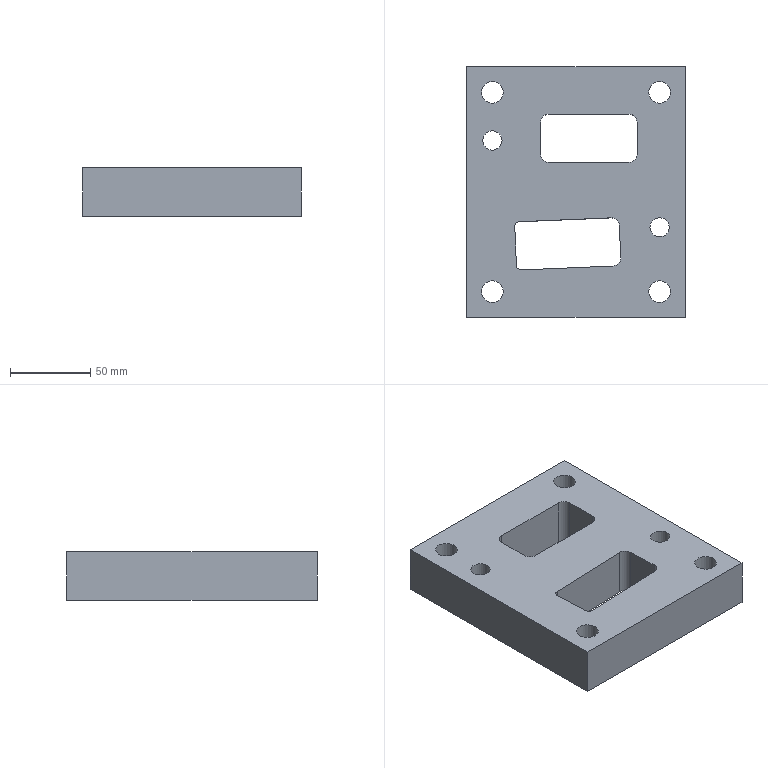Part | NX | features 7 2 | 1 solid | 40 faces | box 136 x 156 x 30 mm | volume 489972 mm3 | plane 20 | cylinder 20 | commonest cylinder face diameters 10 x6 13.5 x4 20 x4 6 x2 12.001 x2 14.11 x2
STEP:
#1=CARTESIAN_POINT('',(3690.489,357.828,91.));
#2=VERTEX_POINT('',#1);
#3=CARTESIAN_POINT('',(3693.361,360.951,91.));
#4=VERTEX_POINT('',#3);
#5=CARTESIAN_POINT('',(3693.487,357.953,91.));
#6=DIRECTION('',(0.,0.,-1.));
#7=DIRECTION('',(1.,0.,0.));
#8=AXIS2_PLACEMENT_3D('',#5,#6,#7);
#9=CIRCLE('',#8,3.);
#10=EDGE_CURVE('',#2,#4,#9,.T.);
#11=ORIENTED_EDGE('',*,*,#10,.T.);
#12=CARTESIAN_POINT('',(3750.311,363.335,91.));
#13=VERTEX_POINT('',#12);
#14=CARTESIAN_POINT('',(3740.376,362.919,91.));
#15=DIRECTION('',(-0.9991,-0.04184,0.));
#16=VECTOR('',#15,1000.);
#17=LINE('',#14,#16);
#18=EDGE_CURVE('',#13,#4,#17,.T.);
#19=ORIENTED_EDGE('',*,*,#18,.F.);
#20=CARTESIAN_POINT('',(3755.516,358.549,91.));
#21=VERTEX_POINT('',#20);
#22=CARTESIAN_POINT('',(3750.52,358.34,91.));
#23=DIRECTION('',(0.,0.,-1.));
#24=DIRECTION('',(1.,0.,0.));
#25=AXIS2_PLACEMENT_3D('',#22,#23,#24);
#26=CIRCLE('',#25,5.);
#27=EDGE_CURVE('',#13,#21,#26,.T.);
#28=ORIENTED_EDGE('',*,*,#27,.T.);
#29=CARTESIAN_POINT('',(3756.353,338.567,91.));
#30=VERTEX_POINT('',#29);
#31=CARTESIAN_POINT('',(3754.595,380.539,91.));
#32=DIRECTION('',(-0.04184,0.9991,0.));
#33=VECTOR('',#32,1000.);
#34=LINE('',#31,#33);
#35=EDGE_CURVE('',#30,#21,#34,.T.);
#36=ORIENTED_EDGE('',*,*,#35,.F.);
#37=CARTESIAN_POINT('',(3751.566,333.362,91.));
#38=VERTEX_POINT('',#37);
#39=CARTESIAN_POINT('',(3751.357,338.357,91.));
#40=DIRECTION('',(0.,0.,-1.));
#41=DIRECTION('',(1.,0.,0.));
#42=AXIS2_PLACEMENT_3D('',#39,#40,#41);
#43=CIRCLE('',#42,5.);
#44=EDGE_CURVE('',#30,#38,#43,.T.);
#45=ORIENTED_EDGE('',*,*,#44,.T.);
#46=CARTESIAN_POINT('',(3694.616,330.977,91.));
#47=VERTEX_POINT('',#46);
#48=CARTESIAN_POINT('',(3741.631,332.946,91.));
#49=DIRECTION('',(0.9991,0.04184,0.));
#50=VECTOR('',#49,1000.);
#51=LINE('',#48,#50);
#52=EDGE_CURVE('',#47,#38,#51,.T.);
#53=ORIENTED_EDGE('',*,*,#52,.F.);
#54=CARTESIAN_POINT('',(3691.493,333.849,91.));
#55=VERTEX_POINT('',#54);
#56=CARTESIAN_POINT('',(3694.491,333.974,91.));
#57=DIRECTION('',(0.,0.,-1.));
#58=DIRECTION('',(1.,0.,0.));
#59=AXIS2_PLACEMENT_3D('',#56,#57,#58);
#60=CIRCLE('',#59,3.);
#61=EDGE_CURVE('',#47,#55,#60,.T.);
#62=ORIENTED_EDGE('',*,*,#61,.T.);
#63=CARTESIAN_POINT('',(3689.652,377.82,91.));
#64=DIRECTION('',(0.04184,-0.9991,0.));
#65=VECTOR('',#64,1000.);
#66=LINE('',#63,#65);
#67=EDGE_CURVE('',#2,#55,#66,.T.);
#68=ORIENTED_EDGE('',*,*,#67,.F.);
#69=EDGE_LOOP('',(#11,#19,#28,#36,#45,#53,#62,#68));
#70=FACE_BOUND('',#69,.T.);
#71=CARTESIAN_POINT('',(3786.562,357.449,91.));
#72=VERTEX_POINT('',#71);
#73=CARTESIAN_POINT('',(3780.562,357.449,91.));
#74=DIRECTION('',(0.,0.,-1.));
#75=DIRECTION('',(1.,0.,0.));
#76=AXIS2_PLACEMENT_3D('',#73,#74,#75);
#77=CIRCLE('',#76,6.);
#78=EDGE_CURVE('',#72,#72,#77,.T.);
#79=ORIENTED_EDGE('',*,*,#78,.T.);
#80=EDGE_LOOP('',(#79));
#81=FACE_BOUND('',#80,.T.);
#82=CARTESIAN_POINT('',(3682.562,411.449,91.));
#83=VERTEX_POINT('',#82);
#84=CARTESIAN_POINT('',(3676.562,411.449,91.));
#85=DIRECTION('',(0.,0.,-1.));
#86=DIRECTION('',(1.,0.,0.));
#87=AXIS2_PLACEMENT_3D('',#84,#85,#86);
#88=CIRCLE('',#87,6.);
#89=EDGE_CURVE('',#83,#83,#88,.T.);
#90=ORIENTED_EDGE('',*,*,#89,.T.);
#91=EDGE_LOOP('',(#90));
#92=FACE_BOUND('',#91,.T.);
#93=CARTESIAN_POINT('',(3683.312,317.449,91.));
#94=VERTEX_POINT('',#93);
#95=CARTESIAN_POINT('',(3676.562,317.449,91.));
#96=DIRECTION('',(0.,0.,-1.));
#97=DIRECTION('',(1.,0.,0.));
#98=AXIS2_PLACEMENT_3D('',#95,#96,#97);
#99=CIRCLE('',#98,6.75);
#100=EDGE_CURVE('',#94,#94,#99,.T.);
#101=ORIENTED_EDGE('',*,*,#100,.T.);
#102=EDGE_LOOP('',(#101));
#103=FACE_BOUND('',#102,.T.);
#104=CARTESIAN_POINT('',(3787.312,441.449,91.));
#105=VERTEX_POINT('',#104);
#106=CARTESIAN_POINT('',(3780.562,441.449,91.));
#107=DIRECTION('',(0.,0.,-1.));
#108=DIRECTION('',(1.,0.,0.));
#109=AXIS2_PLACEMENT_3D('',#106,#107,#108);
#110=CIRCLE('',#109,6.75);
#111=EDGE_CURVE('',#105,#105,#110,.T.);
#112=ORIENTED_EDGE('',*,*,#111,.T.);
#113=EDGE_LOOP('',(#112));
#114=FACE_BOUND('',#113,.T.);
#115=CARTESIAN_POINT('',(3787.312,317.449,91.));
#116=VERTEX_POINT('',#115);
#117=CARTESIAN_POINT('',(3780.562,317.449,91.));
#118=DIRECTION('',(0.,0.,-1.));
#119=DIRECTION('',(1.,0.,0.));
#120=AXIS2_PLACEMENT_3D('',#117,#118,#119);
#121=CIRCLE('',#120,6.75);
#122=EDGE_CURVE('',#116,#116,#121,.T.);
#123=ORIENTED_EDGE('',*,*,#122,.T.);
#124=EDGE_LOOP('',(#123));
#125=FACE_BOUND('',#124,.T.);
#126=CARTESIAN_POINT('',(3683.312,441.449,91.));
#127=VERTEX_POINT('',#126);
#128=CARTESIAN_POINT('',(3676.562,441.449,91.));
#129=DIRECTION('',(0.,0.,-1.));
#130=DIRECTION('',(1.,0.,0.));
#131=AXIS2_PLACEMENT_3D('',#128,#129,#130);
#132=CIRCLE('',#131,6.75);
#133=EDGE_CURVE('',#127,#127,#132,.T.);
#134=ORIENTED_EDGE('',*,*,#133,.T.);
#135=EDGE_LOOP('',(#134));
#136=FACE_BOUND('',#135,.T.);
#137=CARTESIAN_POINT('',(3796.562,457.449,91.));
#138=VERTEX_POINT('',#137);
#139=CARTESIAN_POINT('',(3660.562,457.449,91.));
#140=VERTEX_POINT('',#139);
#141=CARTESIAN_POINT('',(3728.562,457.449,91.));
#142=DIRECTION('',(-1.,0.,0.));
#143=VECTOR('',#142,1000.);
#144=LINE('',#141,#143);
#145=EDGE_CURVE('',#138,#140,#144,.T.);
#146=ORIENTED_EDGE('',*,*,#145,.T.);
#147=CARTESIAN_POINT('',(3660.562,301.449,91.));
#148=VERTEX_POINT('',#147);
#149=CARTESIAN_POINT('',(3660.562,379.449,91.));
#150=DIRECTION('',(0.,-1.,0.));
#151=VECTOR('',#150,1000.);
#152=LINE('',#149,#151);
#153=EDGE_CURVE('',#140,#148,#152,.T.);
#154=ORIENTED_EDGE('',*,*,#153,.T.);
#155=CARTESIAN_POINT('',(3796.562,301.449,91.));
#156=VERTEX_POINT('',#155);
#157=CARTESIAN_POINT('',(3728.562,301.449,91.));
#158=DIRECTION('',(1.,0.,0.));
#159=VECTOR('',#158,1000.);
#160=LINE('',#157,#159);
#161=EDGE_CURVE('',#148,#156,#160,.T.);
#162=ORIENTED_EDGE('',*,*,#161,.T.);
#163=CARTESIAN_POINT('',(3796.562,379.449,91.));
#164=DIRECTION('',(0.,1.,0.));
#165=VECTOR('',#164,1000.);
#166=LINE('',#163,#165);
#167=EDGE_CURVE('',#156,#138,#166,.T.);
#168=ORIENTED_EDGE('',*,*,#167,.T.);
#169=EDGE_LOOP('',(#146,#154,#162,#168));
#170=FACE_BOUND('',#169,.T.);
#171=CARTESIAN_POINT('',(3711.499,397.84,91.));
#172=VERTEX_POINT('',#171);
#173=CARTESIAN_POINT('',(3706.499,402.84,91.));
#174=VERTEX_POINT('',#173);
#175=CARTESIAN_POINT('',(3711.499,402.84,91.));
#176=DIRECTION('',(0.,0.,-1.));
#177=DIRECTION('',(1.,0.,0.));
#178=AXIS2_PLACEMENT_3D('',#175,#176,#177);
#179=CIRCLE('',#178,5.);
#180=EDGE_CURVE('',#172,#174,#179,.T.);
#181=ORIENTED_EDGE('',*,*,#180,.T.);
#182=CARTESIAN_POINT('',(3706.499,422.84,91.));
#183=VERTEX_POINT('',#182);
#184=CARTESIAN_POINT('',(3706.499,412.84,91.));
#185=DIRECTION('',(0.,-1.,0.));
#186=VECTOR('',#185,1000.);
#187=LINE('',#184,#186);
#188=EDGE_CURVE('',#183,#174,#187,.T.);
#189=ORIENTED_EDGE('',*,*,#188,.F.);
#190=CARTESIAN_POINT('',(3711.499,427.84,91.));
#191=VERTEX_POINT('',#190);
#192=CARTESIAN_POINT('',(3711.499,422.84,91.));
#193=DIRECTION('',(0.,0.,-1.));
#194=DIRECTION('',(1.,0.,0.));
#195=AXIS2_PLACEMENT_3D('',#192,#193,#194);
#196=CIRCLE('',#195,5.);
#197=EDGE_CURVE('',#183,#191,#196,.T.);
#198=ORIENTED_EDGE('',*,*,#197,.T.);
#199=CARTESIAN_POINT('',(3761.499,427.84,91.));
#200=VERTEX_POINT('',#199);
#201=CARTESIAN_POINT('',(3721.499,427.84,91.));
#202=DIRECTION('',(-1.,0.,0.));
#203=VECTOR('',#202,1000.);
#204=LINE('',#201,#203);
#205=EDGE_CURVE('',#200,#191,#204,.T.);
#206=ORIENTED_EDGE('',*,*,#205,.F.);
#207=CARTESIAN_POINT('',(3766.499,422.84,91.));
#208=VERTEX_POINT('',#207);
#209=CARTESIAN_POINT('',(3761.499,422.84,91.));
#210=DIRECTION('',(0.,0.,-1.));
#211=DIRECTION('',(1.,0.,0.));
#212=AXIS2_PLACEMENT_3D('',#209,#210,#211);
#213=CIRCLE('',#212,5.);
#214=EDGE_CURVE('',#200,#208,#213,.T.);
#215=ORIENTED_EDGE('',*,*,#214,.T.);
#216=CARTESIAN_POINT('',(3766.499,402.84,91.));
#217=VERTEX_POINT('',#216);
#218=CARTESIAN_POINT('',(3766.499,412.84,91.));
#219=DIRECTION('',(0.,1.,0.));
#220=VECTOR('',#219,1000.);
#221=LINE('',#218,#220);
#222=EDGE_CURVE('',#217,#208,#221,.T.);
#223=ORIENTED_EDGE('',*,*,#222,.F.);
#224=CARTESIAN_POINT('',(3761.499,397.84,91.));
#225=VERTEX_POINT('',#224);
#226=CARTESIAN_POINT('',(3761.499,402.84,91.));
#227=DIRECTION('',(0.,0.,-1.));
#228=DIRECTION('',(1.,0.,0.));
#229=AXIS2_PLACEMENT_3D('',#226,#227,#228);
#230=CIRCLE('',#229,5.);
#231=EDGE_CURVE('',#217,#225,#230,.T.);
#232=ORIENTED_EDGE('',*,*,#231,.T.);
#233=CARTESIAN_POINT('',(3721.499,397.84,91.));
#234=DIRECTION('',(1.,0.,0.));
#235=VECTOR('',#234,1000.);
#236=LINE('',#233,#235);
#237=EDGE_CURVE('',#172,#225,#236,.T.);
#238=ORIENTED_EDGE('',*,*,#237,.F.);
#239=EDGE_LOOP('',(#181,#189,#198,#206,#215,#223,#232,#238));
#240=FACE_BOUND('',#239,.T.);
#241=CARTESIAN_POINT('',(3728.562,379.449,91.));
#242=DIRECTION('',(0.,0.,1.));
#243=DIRECTION('',(-1.,0.,0.));
#244=AXIS2_PLACEMENT_3D('',#241,#242,#243);
#245=PLANE('',#244);
#246=ADVANCED_FACE('',(#70,#81,#92,#103,#114,#125,#136,#170,#240),#245,.T.);
#247=CARTESIAN_POINT('',(3787.617,357.449,61.));
#248=VERTEX_POINT('',#247);
#249=CARTESIAN_POINT('',(3780.562,357.449,61.));
#250=DIRECTION('',(0.,0.,1.));
#251=DIRECTION('',(1.,0.,0.));
#252=AXIS2_PLACEMENT_3D('',#249,#250,#251);
#253=CIRCLE('',#252,7.055);
#254=EDGE_CURVE('',#248,#248,#253,.T.);
#255=ORIENTED_EDGE('',*,*,#254,.T.);
#256=EDGE_LOOP('',(#255));
#257=FACE_BOUND('',#256,.T.);
#258=CARTESIAN_POINT('',(3683.617,411.449,61.));
#259=VERTEX_POINT('',#258);
#260=CARTESIAN_POINT('',(3676.562,411.449,61.));
#261=DIRECTION('',(0.,0.,1.));
#262=DIRECTION('',(1.,0.,0.));
#263=AXIS2_PLACEMENT_3D('',#260,#261,#262);
#264=CIRCLE('',#263,7.055);
#265=EDGE_CURVE('',#259,#259,#264,.T.);
#266=ORIENTED_EDGE('',*,*,#265,.T.);
#267=EDGE_LOOP('',(#266));
#268=FACE_BOUND('',#267,.T.);
#269=CARTESIAN_POINT('',(3750.311,363.335,61.));
#270=VERTEX_POINT('',#269);
#271=CARTESIAN_POINT('',(3693.361,360.951,61.));
#272=VERTEX_POINT('',#271);
#273=CARTESIAN_POINT('',(3729.273,362.454,61.));
#274=DIRECTION('',(-0.9991,-0.04184,0.));
#275=VECTOR('',#274,1000.);
#276=LINE('',#273,#275);
#277=EDGE_CURVE('',#270,#272,#276,.T.);
#278=ORIENTED_EDGE('',*,*,#277,.T.);
#279=CARTESIAN_POINT('',(3690.489,357.828,61.));
#280=VERTEX_POINT('',#279);
#281=CARTESIAN_POINT('',(3693.487,357.953,61.));
#282=DIRECTION('',(0.,0.,-1.));
#283=DIRECTION('',(-1.,0.,0.));
#284=AXIS2_PLACEMENT_3D('',#281,#282,#283);
#285=CIRCLE('',#284,3.);
#286=EDGE_CURVE('',#280,#272,#285,.T.);
#287=ORIENTED_EDGE('',*,*,#286,.F.);
#288=CARTESIAN_POINT('',(3691.493,333.849,61.));
#289=VERTEX_POINT('',#288);
#290=CARTESIAN_POINT('',(3690.991,345.838,61.));
#291=DIRECTION('',(0.04184,-0.9991,0.));
#292=VECTOR('',#291,1000.);
#293=LINE('',#290,#292);
#294=EDGE_CURVE('',#280,#289,#293,.T.);
#295=ORIENTED_EDGE('',*,*,#294,.T.);
#296=CARTESIAN_POINT('',(3694.616,330.977,61.));
#297=VERTEX_POINT('',#296);
#298=CARTESIAN_POINT('',(3694.491,333.974,61.));
#299=DIRECTION('',(0.,0.,-1.));
#300=DIRECTION('',(-1.,0.,0.));
#301=AXIS2_PLACEMENT_3D('',#298,#299,#300);
#302=CIRCLE('',#301,3.);
#303=EDGE_CURVE('',#297,#289,#302,.T.);
#304=ORIENTED_EDGE('',*,*,#303,.F.);
#305=CARTESIAN_POINT('',(3751.566,333.362,61.));
#306=VERTEX_POINT('',#305);
#307=CARTESIAN_POINT('',(3730.528,332.481,61.));
#308=DIRECTION('',(0.9991,0.04184,0.));
#309=VECTOR('',#308,1000.);
#310=LINE('',#307,#309);
#311=EDGE_CURVE('',#297,#306,#310,.T.);
#312=ORIENTED_EDGE('',*,*,#311,.T.);
#313=CARTESIAN_POINT('',(3756.353,338.567,61.));
#314=VERTEX_POINT('',#313);
#315=CARTESIAN_POINT('',(3751.357,338.357,61.));
#316=DIRECTION('',(0.,0.,1.));
#317=DIRECTION('',(-1.,0.,0.));
#318=AXIS2_PLACEMENT_3D('',#315,#316,#317);
#319=CIRCLE('',#318,5.);
#320=EDGE_CURVE('',#306,#314,#319,.T.);
#321=ORIENTED_EDGE('',*,*,#320,.T.);
#322=CARTESIAN_POINT('',(3755.516,358.549,61.));
#323=VERTEX_POINT('',#322);
#324=CARTESIAN_POINT('',(3755.934,348.558,61.));
#325=DIRECTION('',(-0.04184,0.9991,0.));
#326=VECTOR('',#325,1000.);
#327=LINE('',#324,#326);
#328=EDGE_CURVE('',#314,#323,#327,.T.);
#329=ORIENTED_EDGE('',*,*,#328,.T.);
#330=CARTESIAN_POINT('',(3750.52,358.34,61.));
#331=DIRECTION('',(0.,0.,1.));
#332=DIRECTION('',(-1.,0.,0.));
#333=AXIS2_PLACEMENT_3D('',#330,#331,#332);
#334=CIRCLE('',#333,5.);
#335=EDGE_CURVE('',#323,#270,#334,.T.);
#336=ORIENTED_EDGE('',*,*,#335,.T.);
#337=EDGE_LOOP('',(#278,#287,#295,#304,#312,#321,#329,#336));
#338=FACE_BOUND('',#337,.T.);
#339=CARTESIAN_POINT('',(3761.499,397.84,61.));
#340=VERTEX_POINT('',#339);
#341=CARTESIAN_POINT('',(3766.499,402.84,61.));
#342=VERTEX_POINT('',#341);
#343=CARTESIAN_POINT('',(3761.499,402.84,61.));
#344=DIRECTION('',(0.,0.,1.));
#345=DIRECTION('',(-1.,0.,0.));
#346=AXIS2_PLACEMENT_3D('',#343,#344,#345);
#347=CIRCLE('',#346,5.);
#348=EDGE_CURVE('',#340,#342,#347,.T.);
#349=ORIENTED_EDGE('',*,*,#348,.T.);
#350=CARTESIAN_POINT('',(3766.499,422.84,61.));
#351=VERTEX_POINT('',#350);
#352=CARTESIAN_POINT('',(3766.499,379.449,61.));
#353=DIRECTION('',(0.,1.,0.));
#354=VECTOR('',#353,1000.);
#355=LINE('',#352,#354);
#356=EDGE_CURVE('',#342,#351,#355,.T.);
#357=ORIENTED_EDGE('',*,*,#356,.T.);
#358=CARTESIAN_POINT('',(3761.499,427.84,61.));
#359=VERTEX_POINT('',#358);
#360=CARTESIAN_POINT('',(3761.499,422.84,61.));
#361=DIRECTION('',(0.,0.,1.));
#362=DIRECTION('',(-1.,0.,0.));
#363=AXIS2_PLACEMENT_3D('',#360,#361,#362);
#364=CIRCLE('',#363,5.);
#365=EDGE_CURVE('',#351,#359,#364,.T.);
#366=ORIENTED_EDGE('',*,*,#365,.T.);
#367=CARTESIAN_POINT('',(3711.499,427.84,61.));
#368=VERTEX_POINT('',#367);
#369=CARTESIAN_POINT('',(3728.562,427.84,61.));
#370=DIRECTION('',(-1.,0.,0.));
#371=VECTOR('',#370,1000.);
#372=LINE('',#369,#371);
#373=EDGE_CURVE('',#359,#368,#372,.T.);
#374=ORIENTED_EDGE('',*,*,#373,.T.);
#375=CARTESIAN_POINT('',(3706.499,422.84,61.));
#376=VERTEX_POINT('',#375);
#377=CARTESIAN_POINT('',(3711.499,422.84,61.));
#378=DIRECTION('',(0.,0.,1.));
#379=DIRECTION('',(-1.,0.,0.));
#380=AXIS2_PLACEMENT_3D('',#377,#378,#379);
#381=CIRCLE('',#380,5.);
#382=EDGE_CURVE('',#368,#376,#381,.T.);
#383=ORIENTED_EDGE('',*,*,#382,.T.);
#384=CARTESIAN_POINT('',(3706.499,402.84,61.));
#385=VERTEX_POINT('',#384);
#386=CARTESIAN_POINT('',(3706.499,379.449,61.));
#387=DIRECTION('',(0.,-1.,0.));
#388=VECTOR('',#387,1000.);
#389=LINE('',#386,#388);
#390=EDGE_CURVE('',#376,#385,#389,.T.);
#391=ORIENTED_EDGE('',*,*,#390,.T.);
#392=CARTESIAN_POINT('',(3711.499,397.84,61.));
#393=VERTEX_POINT('',#392);
#394=CARTESIAN_POINT('',(3711.499,402.84,61.));
#395=DIRECTION('',(0.,0.,1.));
#396=DIRECTION('',(-1.,0.,0.));
#397=AXIS2_PLACEMENT_3D('',#394,#395,#396);
#398=CIRCLE('',#397,5.);
#399=EDGE_CURVE('',#385,#393,#398,.T.);
#400=ORIENTED_EDGE('',*,*,#399,.T.);
#401=CARTESIAN_POINT('',(3728.562,397.84,61.));
#402=DIRECTION('',(1.,0.,0.));
#403=VECTOR('',#402,1000.);
#404=LINE('',#401,#403);
#405=EDGE_CURVE('',#393,#340,#404,.T.);
#406=ORIENTED_EDGE('',*,*,#405,.T.);
#407=EDGE_LOOP('',(#349,#357,#366,#374,#383,#391,#400,#406));
#408=FACE_BOUND('',#407,.T.);
#409=CARTESIAN_POINT('',(3790.562,441.449,61.));
#410=VERTEX_POINT('',#409);
#411=CARTESIAN_POINT('',(3780.562,441.449,61.));
#412=DIRECTION('',(0.,0.,-1.));
#413=DIRECTION('',(1.,0.,0.));
#414=AXIS2_PLACEMENT_3D('',#411,#412,#413);
#415=CIRCLE('',#414,10.);
#416=EDGE_CURVE('',#410,#410,#415,.T.);
#417=ORIENTED_EDGE('',*,*,#416,.F.);
#418=EDGE_LOOP('',(#417));
#419=FACE_BOUND('',#418,.T.);
#420=CARTESIAN_POINT('',(3686.562,441.449,61.));
#421=VERTEX_POINT('',#420);
#422=CARTESIAN_POINT('',(3676.562,441.449,61.));
#423=DIRECTION('',(0.,0.,-1.));
#424=DIRECTION('',(1.,0.,0.));
#425=AXIS2_PLACEMENT_3D('',#422,#423,#424);
#426=CIRCLE('',#425,10.);
#427=EDGE_CURVE('',#421,#421,#426,.T.);
#428=ORIENTED_EDGE('',*,*,#427,.F.);
#429=EDGE_LOOP('',(#428));
#430=FACE_BOUND('',#429,.T.);
#431=CARTESIAN_POINT('',(3796.562,457.449,61.));
#432=VERTEX_POINT('',#431);
#433=CARTESIAN_POINT('',(3796.562,301.449,61.));
#434=VERTEX_POINT('',#433);
#435=CARTESIAN_POINT('',(3796.562,379.449,61.));
#436=DIRECTION('',(0.,-1.,0.));
#437=VECTOR('',#436,1000.);
#438=LINE('',#435,#437);
#439=EDGE_CURVE('',#432,#434,#438,.T.);
#440=ORIENTED_EDGE('',*,*,#439,.T.);
#441=CARTESIAN_POINT('',(3660.562,301.449,61.));
#442=VERTEX_POINT('',#441);
#443=CARTESIAN_POINT('',(3728.562,301.449,61.));
#444=DIRECTION('',(-1.,0.,0.));
#445=VECTOR('',#444,1000.);
#446=LINE('',#443,#445);
#447=EDGE_CURVE('',#434,#442,#446,.T.);
#448=ORIENTED_EDGE('',*,*,#447,.T.);
#449=CARTESIAN_POINT('',(3660.562,457.449,61.));
#450=VERTEX_POINT('',#449);
#451=CARTESIAN_POINT('',(3660.562,379.449,61.));
#452=DIRECTION('',(0.,1.,0.));
#453=VECTOR('',#452,1000.);
#454=LINE('',#451,#453);
#455=EDGE_CURVE('',#442,#450,#454,.T.);
#456=ORIENTED_EDGE('',*,*,#455,.T.);
#457=CARTESIAN_POINT('',(3728.562,457.449,61.));
#458=DIRECTION('',(1.,0.,0.));
#459=VECTOR('',#458,1000.);
#460=LINE('',#457,#459);
#461=EDGE_CURVE('',#450,#432,#460,.T.);
#462=ORIENTED_EDGE('',*,*,#461,.T.);
#463=EDGE_LOOP('',(#440,#448,#456,#462));
#464=FACE_BOUND('',#463,.T.);
#465=CARTESIAN_POINT('',(3790.562,317.449,61.));
#466=VERTEX_POINT('',#465);
#467=CARTESIAN_POINT('',(3780.562,317.449,61.));
#468=DIRECTION('',(0.,0.,-1.));
#469=DIRECTION('',(1.,0.,0.));
#470=AXIS2_PLACEMENT_3D('',#467,#468,#469);
#471=CIRCLE('',#470,10.);
#472=EDGE_CURVE('',#466,#466,#471,.T.);
#473=ORIENTED_EDGE('',*,*,#472,.F.);
#474=EDGE_LOOP('',(#473));
#475=FACE_BOUND('',#474,.T.);
#476=CARTESIAN_POINT('',(3686.562,317.449,61.));
#477=VERTEX_POINT('',#476);
#478=CARTESIAN_POINT('',(3676.562,317.449,61.));
#479=DIRECTION('',(0.,0.,-1.));
#480=DIRECTION('',(1.,0.,0.));
#481=AXIS2_PLACEMENT_3D('',#478,#479,#480);
#482=CIRCLE('',#481,10.);
#483=EDGE_CURVE('',#477,#477,#482,.T.);
#484=ORIENTED_EDGE('',*,*,#483,.F.);
#485=EDGE_LOOP('',(#484));
#486=FACE_BOUND('',#485,.T.);
#487=CARTESIAN_POINT('',(3728.562,379.449,61.));
#488=DIRECTION('',(0.,0.,-1.));
#489=DIRECTION('',(1.,0.,0.));
#490=AXIS2_PLACEMENT_3D('',#487,#488,#489);
#491=PLANE('',#490);
#492=ADVANCED_FACE('',(#257,#268,#338,#408,#419,#430,#464,#475,#486),#491,.T.);
#493=CARTESIAN_POINT('',(3796.562,457.449,61.));
#494=DIRECTION('',(0.,0.,1.));
#495=VECTOR('',#494,1000.);
#496=LINE('',#493,#495);
#497=EDGE_CURVE('',#432,#138,#496,.T.);
#498=ORIENTED_EDGE('',*,*,#497,.F.);
#499=ORIENTED_EDGE('',*,*,#461,.F.);
#500=CARTESIAN_POINT('',(3660.562,457.449,61.));
#501=DIRECTION('',(0.,0.,1.));
#502=VECTOR('',#501,1000.);
#503=LINE('',#500,#502);
#504=EDGE_CURVE('',#450,#140,#503,.T.);
#505=ORIENTED_EDGE('',*,*,#504,.T.);
#506=ORIENTED_EDGE('',*,*,#145,.F.);
#507=EDGE_LOOP('',(#498,#499,#505,#506));
#508=FACE_BOUND('',#507,.T.);
#509=CARTESIAN_POINT('',(3728.562,457.449,61.));
#510=DIRECTION('',(0.,1.,0.));
#511=DIRECTION('',(0.,0.,1.));
#512=AXIS2_PLACEMENT_3D('',#509,#510,#511);
#513=PLANE('',#512);
#514=ADVANCED_FACE('',(#508),#513,.T.);
#515=ORIENTED_EDGE('',*,*,#504,.F.);
#516=ORIENTED_EDGE('',*,*,#455,.F.);
#517=CARTESIAN_POINT('',(3660.562,301.449,61.));
#518=DIRECTION('',(0.,0.,1.));
#519=VECTOR('',#518,1000.);
#520=LINE('',#517,#519);
#521=EDGE_CURVE('',#442,#148,#520,.T.);
#522=ORIENTED_EDGE('',*,*,#521,.T.);
#523=ORIENTED_EDGE('',*,*,#153,.F.);
#524=EDGE_LOOP('',(#515,#516,#522,#523));
#525=FACE_BOUND('',#524,.T.);
#526=CARTESIAN_POINT('',(3660.562,379.449,61.));
#527=DIRECTION('',(-1.,0.,0.));
#528=DIRECTION('',(0.,0.,-1.));
#529=AXIS2_PLACEMENT_3D('',#526,#527,#528);
#530=PLANE('',#529);
#531=ADVANCED_FACE('',(#525),#530,.T.);
#532=ORIENTED_EDGE('',*,*,#521,.F.);
#533=ORIENTED_EDGE('',*,*,#447,.F.);
#534=CARTESIAN_POINT('',(3796.562,301.449,61.));
#535=DIRECTION('',(0.,0.,1.));
#536=VECTOR('',#535,1000.);
#537=LINE('',#534,#536);
#538=EDGE_CURVE('',#434,#156,#537,.T.);
#539=ORIENTED_EDGE('',*,*,#538,.T.);
#540=ORIENTED_EDGE('',*,*,#161,.F.);
#541=EDGE_LOOP('',(#532,#533,#539,#540));
#542=FACE_BOUND('',#541,.T.);
#543=CARTESIAN_POINT('',(3728.562,301.449,61.));
#544=DIRECTION('',(0.,-1.,0.));
#545=DIRECTION('',(0.,0.,-1.));
#546=AXIS2_PLACEMENT_3D('',#543,#544,#545);
#547=PLANE('',#546);
#548=ADVANCED_FACE('',(#542),#547,.T.);
#549=ORIENTED_EDGE('',*,*,#439,.F.);
#550=ORIENTED_EDGE('',*,*,#497,.T.);
#551=ORIENTED_EDGE('',*,*,#167,.F.);
#552=ORIENTED_EDGE('',*,*,#538,.F.);
#553=EDGE_LOOP('',(#549,#550,#551,#552));
#554=FACE_BOUND('',#553,.T.);
#555=CARTESIAN_POINT('',(3796.562,379.449,61.));
#556=DIRECTION('',(1.,0.,0.));
#557=DIRECTION('',(0.,0.,1.));
#558=AXIS2_PLACEMENT_3D('',#555,#556,#557);
#559=PLANE('',#558);
#560=ADVANCED_FACE('',(#554),#559,.T.);
#561=ORIENTED_EDGE('',*,*,#133,.F.);
#562=EDGE_LOOP('',(#561));
#563=FACE_BOUND('',#562,.T.);
#564=CARTESIAN_POINT('',(3683.312,441.449,76.));
#565=VERTEX_POINT('',#564);
#566=CARTESIAN_POINT('',(3676.562,441.449,76.));
#567=DIRECTION('',(0.,0.,-1.));
#568=DIRECTION('',(1.,0.,0.));
#569=AXIS2_PLACEMENT_3D('',#566,#567,#568);
#570=CIRCLE('',#569,6.75);
#571=EDGE_CURVE('',#565,#565,#570,.T.);
#572=ORIENTED_EDGE('',*,*,#571,.T.);
#573=EDGE_LOOP('',(#572));
#574=FACE_BOUND('',#573,.T.);
#575=CARTESIAN_POINT('',(3676.562,441.449,58.));
#576=DIRECTION('',(0.,0.,1.));
#577=DIRECTION('',(-1.,0.,0.));
#578=AXIS2_PLACEMENT_3D('',#575,#576,#577);
#579=CYLINDRICAL_SURFACE('',#578,6.75);
#580=ADVANCED_FACE('',(#563,#574),#579,.F.);
#581=ORIENTED_EDGE('',*,*,#571,.F.);
#582=EDGE_LOOP('',(#581));
#583=FACE_BOUND('',#582,.T.);
#584=CARTESIAN_POINT('',(3686.562,441.449,76.));
#585=VERTEX_POINT('',#584);
#586=CARTESIAN_POINT('',(3676.562,441.449,76.));
#587=DIRECTION('',(0.,0.,-1.));
#588=DIRECTION('',(1.,0.,0.));
#589=AXIS2_PLACEMENT_3D('',#586,#587,#588);
#590=CIRCLE('',#589,10.);
#591=EDGE_CURVE('',#585,#585,#590,.T.);
#592=ORIENTED_EDGE('',*,*,#591,.T.);
#593=EDGE_LOOP('',(#592));
#594=FACE_BOUND('',#593,.T.);
#595=CARTESIAN_POINT('',(3676.562,441.449,76.));
#596=DIRECTION('',(0.,0.,1.));
#597=DIRECTION('',(-1.,0.,0.));
#598=AXIS2_PLACEMENT_3D('',#595,#596,#597);
#599=PLANE('',#598);
#600=ADVANCED_FACE('',(#583,#594),#599,.F.);
#601=ORIENTED_EDGE('',*,*,#591,.F.);
#602=EDGE_LOOP('',(#601));
#603=FACE_BOUND('',#602,.T.);
#604=ORIENTED_EDGE('',*,*,#427,.T.);
#605=EDGE_LOOP('',(#604));
#606=FACE_BOUND('',#605,.T.);
#607=CARTESIAN_POINT('',(3676.562,441.449,61.));
#608=DIRECTION('',(0.,0.,1.));
#609=DIRECTION('',(-1.,0.,0.));
#610=AXIS2_PLACEMENT_3D('',#607,#608,#609);
#611=CYLINDRICAL_SURFACE('',#610,10.);
#612=ADVANCED_FACE('',(#603,#606),#611,.F.);
#613=ORIENTED_EDGE('',*,*,#122,.F.);
#614=EDGE_LOOP('',(#613));
#615=FACE_BOUND('',#614,.T.);
#616=CARTESIAN_POINT('',(3787.312,317.449,76.));
#617=VERTEX_POINT('',#616);
#618=CARTESIAN_POINT('',(3780.562,317.449,76.));
#619=DIRECTION('',(0.,0.,-1.));
#620=DIRECTION('',(1.,0.,0.));
#621=AXIS2_PLACEMENT_3D('',#618,#619,#620);
#622=CIRCLE('',#621,6.75);
#623=EDGE_CURVE('',#617,#617,#622,.T.);
#624=ORIENTED_EDGE('',*,*,#623,.T.);
#625=EDGE_LOOP('',(#624));
#626=FACE_BOUND('',#625,.T.);
#627=CARTESIAN_POINT('',(3780.562,317.449,58.));
#628=DIRECTION('',(0.,0.,1.));
#629=DIRECTION('',(-1.,0.,0.));
#630=AXIS2_PLACEMENT_3D('',#627,#628,#629);
#631=CYLINDRICAL_SURFACE('',#630,6.75);
#632=ADVANCED_FACE('',(#615,#626),#631,.F.);
#633=ORIENTED_EDGE('',*,*,#623,.F.);
#634=EDGE_LOOP('',(#633));
#635=FACE_BOUND('',#634,.T.);
#636=CARTESIAN_POINT('',(3790.562,317.449,76.));
#637=VERTEX_POINT('',#636);
#638=CARTESIAN_POINT('',(3780.562,317.449,76.));
#639=DIRECTION('',(0.,0.,-1.));
#640=DIRECTION('',(1.,0.,0.));
#641=AXIS2_PLACEMENT_3D('',#638,#639,#640);
#642=CIRCLE('',#641,10.);
#643=EDGE_CURVE('',#637,#637,#642,.T.);
#644=ORIENTED_EDGE('',*,*,#643,.T.);
#645=EDGE_LOOP('',(#644));
#646=FACE_BOUND('',#645,.T.);
#647=CARTESIAN_POINT('',(3780.562,317.449,76.));
#648=DIRECTION('',(0.,0.,1.));
#649=DIRECTION('',(-1.,0.,0.));
#650=AXIS2_PLACEMENT_3D('',#647,#648,#649);
#651=PLANE('',#650);
#652=ADVANCED_FACE('',(#635,#646),#651,.F.);
#653=ORIENTED_EDGE('',*,*,#643,.F.);
#654=EDGE_LOOP('',(#653));
#655=FACE_BOUND('',#654,.T.);
#656=ORIENTED_EDGE('',*,*,#472,.T.);
#657=EDGE_LOOP('',(#656));
#658=FACE_BOUND('',#657,.T.);
#659=CARTESIAN_POINT('',(3780.562,317.449,61.));
#660=DIRECTION('',(0.,0.,1.));
#661=DIRECTION('',(-1.,0.,0.));
#662=AXIS2_PLACEMENT_3D('',#659,#660,#661);
#663=CYLINDRICAL_SURFACE('',#662,10.);
#664=ADVANCED_FACE('',(#655,#658),#663,.F.);
#665=ORIENTED_EDGE('',*,*,#111,.F.);
#666=EDGE_LOOP('',(#665));
#667=FACE_BOUND('',#666,.T.);
#668=CARTESIAN_POINT('',(3787.312,441.449,76.));
#669=VERTEX_POINT('',#668);
#670=CARTESIAN_POINT('',(3780.562,441.449,76.));
#671=DIRECTION('',(0.,0.,-1.));
#672=DIRECTION('',(1.,0.,0.));
#673=AXIS2_PLACEMENT_3D('',#670,#671,#672);
#674=CIRCLE('',#673,6.75);
#675=EDGE_CURVE('',#669,#669,#674,.T.);
#676=ORIENTED_EDGE('',*,*,#675,.T.);
#677=EDGE_LOOP('',(#676));
#678=FACE_BOUND('',#677,.T.);
#679=CARTESIAN_POINT('',(3780.562,441.449,58.));
#680=DIRECTION('',(0.,0.,1.));
#681=DIRECTION('',(-1.,0.,0.));
#682=AXIS2_PLACEMENT_3D('',#679,#680,#681);
#683=CYLINDRICAL_SURFACE('',#682,6.75);
#684=ADVANCED_FACE('',(#667,#678),#683,.F.);
#685=ORIENTED_EDGE('',*,*,#675,.F.);
#686=EDGE_LOOP('',(#685));
#687=FACE_BOUND('',#686,.T.);
#688=CARTESIAN_POINT('',(3790.562,441.449,76.));
#689=VERTEX_POINT('',#688);
#690=CARTESIAN_POINT('',(3780.562,441.449,76.));
#691=DIRECTION('',(0.,0.,-1.));
#692=DIRECTION('',(1.,0.,0.));
#693=AXIS2_PLACEMENT_3D('',#690,#691,#692);
#694=CIRCLE('',#693,10.);
#695=EDGE_CURVE('',#689,#689,#694,.T.);
#696=ORIENTED_EDGE('',*,*,#695,.T.);
#697=EDGE_LOOP('',(#696));
#698=FACE_BOUND('',#697,.T.);
#699=CARTESIAN_POINT('',(3780.562,441.449,76.));
#700=DIRECTION('',(0.,0.,1.));
#701=DIRECTION('',(-1.,0.,0.));
#702=AXIS2_PLACEMENT_3D('',#699,#700,#701);
#703=PLANE('',#702);
#704=ADVANCED_FACE('',(#687,#698),#703,.F.);
#705=ORIENTED_EDGE('',*,*,#695,.F.);
#706=EDGE_LOOP('',(#705));
#707=FACE_BOUND('',#706,.T.);
#708=ORIENTED_EDGE('',*,*,#416,.T.);
#709=EDGE_LOOP('',(#708));
#710=FACE_BOUND('',#709,.T.);
#711=CARTESIAN_POINT('',(3780.562,441.449,61.));
#712=DIRECTION('',(0.,0.,1.));
#713=DIRECTION('',(-1.,0.,0.));
#714=AXIS2_PLACEMENT_3D('',#711,#712,#713);
#715=CYLINDRICAL_SURFACE('',#714,10.);
#716=ADVANCED_FACE('',(#707,#710),#715,.F.);
#717=ORIENTED_EDGE('',*,*,#100,.F.);
#718=EDGE_LOOP('',(#717));
#719=FACE_BOUND('',#718,.T.);
#720=CARTESIAN_POINT('',(3683.312,317.449,76.));
#721=VERTEX_POINT('',#720);
#722=CARTESIAN_POINT('',(3676.562,317.449,76.));
#723=DIRECTION('',(0.,0.,-1.));
#724=DIRECTION('',(1.,0.,0.));
#725=AXIS2_PLACEMENT_3D('',#722,#723,#724);
#726=CIRCLE('',#725,6.75);
#727=EDGE_CURVE('',#721,#721,#726,.T.);
#728=ORIENTED_EDGE('',*,*,#727,.T.);
#729=EDGE_LOOP('',(#728));
#730=FACE_BOUND('',#729,.T.);
#731=CARTESIAN_POINT('',(3676.562,317.449,58.));
#732=DIRECTION('',(0.,0.,1.));
#733=DIRECTION('',(-1.,0.,0.));
#734=AXIS2_PLACEMENT_3D('',#731,#732,#733);
#735=CYLINDRICAL_SURFACE('',#734,6.75);
#736=ADVANCED_FACE('',(#719,#730),#735,.F.);
#737=ORIENTED_EDGE('',*,*,#727,.F.);
#738=EDGE_LOOP('',(#737));
#739=FACE_BOUND('',#738,.T.);
#740=CARTESIAN_POINT('',(3686.562,317.449,76.));
#741=VERTEX_POINT('',#740);
#742=CARTESIAN_POINT('',(3676.562,317.449,76.));
#743=DIRECTION('',(0.,0.,-1.));
#744=DIRECTION('',(1.,0.,0.));
#745=AXIS2_PLACEMENT_3D('',#742,#743,#744);
#746=CIRCLE('',#745,10.);
#747=EDGE_CURVE('',#741,#741,#746,.T.);
#748=ORIENTED_EDGE('',*,*,#747,.T.);
#749=EDGE_LOOP('',(#748));
#750=FACE_BOUND('',#749,.T.);
#751=CARTESIAN_POINT('',(3676.562,317.449,76.));
#752=DIRECTION('',(0.,0.,1.));
#753=DIRECTION('',(-1.,0.,0.));
#754=AXIS2_PLACEMENT_3D('',#751,#752,#753);
#755=PLANE('',#754);
#756=ADVANCED_FACE('',(#739,#750),#755,.F.);
#757=ORIENTED_EDGE('',*,*,#747,.F.);
#758=EDGE_LOOP('',(#757));
#759=FACE_BOUND('',#758,.T.);
#760=ORIENTED_EDGE('',*,*,#483,.T.);
#761=EDGE_LOOP('',(#760));
#762=FACE_BOUND('',#761,.T.);
#763=CARTESIAN_POINT('',(3676.562,317.449,61.));
#764=DIRECTION('',(0.,0.,1.));
#765=DIRECTION('',(-1.,0.,0.));
#766=AXIS2_PLACEMENT_3D('',#763,#764,#765);
#767=CYLINDRICAL_SURFACE('',#766,10.);
#768=ADVANCED_FACE('',(#759,#762),#767,.F.);
#769=CARTESIAN_POINT('',(3682.562,411.449,71.));
#770=VERTEX_POINT('',#769);
#771=CARTESIAN_POINT('',(3676.562,411.449,71.));
#772=DIRECTION('',(0.,0.,-1.));
#773=DIRECTION('',(1.,0.,0.));
#774=AXIS2_PLACEMENT_3D('',#771,#772,#773);
#775=CIRCLE('',#774,6.);
#776=EDGE_CURVE('',#770,#770,#775,.T.);
#777=ORIENTED_EDGE('',*,*,#776,.T.);
#778=EDGE_LOOP('',(#777));
#779=FACE_BOUND('',#778,.T.);
#780=ORIENTED_EDGE('',*,*,#89,.F.);
#781=EDGE_LOOP('',(#780));
#782=FACE_BOUND('',#781,.T.);
#783=CARTESIAN_POINT('',(3676.562,411.449,58.));
#784=DIRECTION('',(0.,0.,1.));
#785=DIRECTION('',(-1.,0.,0.));
#786=AXIS2_PLACEMENT_3D('',#783,#784,#785);
#787=CYLINDRICAL_SURFACE('',#786,6.);
#788=ADVANCED_FACE('',(#779,#782),#787,.F.);
#789=CARTESIAN_POINT('',(3786.562,357.449,71.));
#790=VERTEX_POINT('',#789);
#791=CARTESIAN_POINT('',(3780.562,357.449,71.));
#792=DIRECTION('',(0.,0.,-1.));
#793=DIRECTION('',(1.,0.,0.));
#794=AXIS2_PLACEMENT_3D('',#791,#792,#793);
#795=CIRCLE('',#794,6.);
#796=EDGE_CURVE('',#790,#790,#795,.T.);
#797=ORIENTED_EDGE('',*,*,#796,.T.);
#798=EDGE_LOOP('',(#797));
#799=FACE_BOUND('',#798,.T.);
#800=ORIENTED_EDGE('',*,*,#78,.F.);
#801=EDGE_LOOP('',(#800));
#802=FACE_BOUND('',#801,.T.);
#803=CARTESIAN_POINT('',(3780.562,357.449,58.));
#804=DIRECTION('',(0.,0.,1.));
#805=DIRECTION('',(-1.,0.,0.));
#806=AXIS2_PLACEMENT_3D('',#803,#804,#805);
#807=CYLINDRICAL_SURFACE('',#806,6.);
#808=ADVANCED_FACE('',(#799,#802),#807,.F.);
#809=ORIENTED_EDGE('',*,*,#365,.F.);
#810=CARTESIAN_POINT('',(3766.499,422.84,-9.));
#811=DIRECTION('',(0.,0.,1.));
#812=VECTOR('',#811,1000.);
#813=LINE('',#810,#812);
#814=EDGE_CURVE('',#351,#208,#813,.T.);
#815=ORIENTED_EDGE('',*,*,#814,.T.);
#816=ORIENTED_EDGE('',*,*,#214,.F.);
#817=CARTESIAN_POINT('',(3761.499,427.84,-9.));
#818=DIRECTION('',(0.,0.,-1.));
#819=VECTOR('',#818,1000.);
#820=LINE('',#817,#819);
#821=EDGE_CURVE('',#200,#359,#820,.T.);
#822=ORIENTED_EDGE('',*,*,#821,.T.);
#823=EDGE_LOOP('',(#809,#815,#816,#822));
#824=FACE_BOUND('',#823,.T.);
#825=CARTESIAN_POINT('',(3761.499,422.84,-9.));
#826=DIRECTION('',(0.,0.,1.));
#827=DIRECTION('',(-1.,0.,0.));
#828=AXIS2_PLACEMENT_3D('',#825,#826,#827);
#829=CYLINDRICAL_SURFACE('',#828,5.);
#830=ADVANCED_FACE('',(#824),#829,.F.);
#831=ORIENTED_EDGE('',*,*,#348,.F.);
#832=CARTESIAN_POINT('',(3761.499,397.84,-9.));
#833=DIRECTION('',(0.,0.,1.));
#834=VECTOR('',#833,1000.);
#835=LINE('',#832,#834);
#836=EDGE_CURVE('',#340,#225,#835,.T.);
#837=ORIENTED_EDGE('',*,*,#836,.T.);
#838=ORIENTED_EDGE('',*,*,#231,.F.);
#839=CARTESIAN_POINT('',(3766.499,402.84,-9.));
#840=DIRECTION('',(0.,0.,-1.));
#841=VECTOR('',#840,1000.);
#842=LINE('',#839,#841);
#843=EDGE_CURVE('',#217,#342,#842,.T.);
#844=ORIENTED_EDGE('',*,*,#843,.T.);
#845=EDGE_LOOP('',(#831,#837,#838,#844));
#846=FACE_BOUND('',#845,.T.);
#847=CARTESIAN_POINT('',(3761.499,402.84,-9.));
#848=DIRECTION('',(0.,0.,1.));
#849=DIRECTION('',(-1.,0.,0.));
#850=AXIS2_PLACEMENT_3D('',#847,#848,#849);
#851=CYLINDRICAL_SURFACE('',#850,5.);
#852=ADVANCED_FACE('',(#846),#851,.F.);
#853=ORIENTED_EDGE('',*,*,#356,.F.);
#854=ORIENTED_EDGE('',*,*,#843,.F.);
#855=ORIENTED_EDGE('',*,*,#222,.T.);
#856=ORIENTED_EDGE('',*,*,#814,.F.);
#857=EDGE_LOOP('',(#853,#854,#855,#856));
#858=FACE_BOUND('',#857,.T.);
#859=CARTESIAN_POINT('',(3766.499,412.84,-9.));
#860=DIRECTION('',(1.,0.,0.));
#861=DIRECTION('',(0.,0.,1.));
#862=AXIS2_PLACEMENT_3D('',#859,#860,#861);
#863=PLANE('',#862);
#864=ADVANCED_FACE('',(#858),#863,.F.);
#865=ORIENTED_EDGE('',*,*,#399,.F.);
#866=CARTESIAN_POINT('',(3706.499,402.84,-9.));
#867=DIRECTION('',(0.,0.,1.));
#868=VECTOR('',#867,1000.);
#869=LINE('',#866,#868);
#870=EDGE_CURVE('',#385,#174,#869,.T.);
#871=ORIENTED_EDGE('',*,*,#870,.T.);
#872=ORIENTED_EDGE('',*,*,#180,.F.);
#873=CARTESIAN_POINT('',(3711.499,397.84,-9.));
#874=DIRECTION('',(0.,0.,-1.));
#875=VECTOR('',#874,1000.);
#876=LINE('',#873,#875);
#877=EDGE_CURVE('',#172,#393,#876,.T.);
#878=ORIENTED_EDGE('',*,*,#877,.T.);
#879=EDGE_LOOP('',(#865,#871,#872,#878));
#880=FACE_BOUND('',#879,.T.);
#881=CARTESIAN_POINT('',(3711.499,402.84,-9.));
#882=DIRECTION('',(0.,0.,1.));
#883=DIRECTION('',(-1.,0.,0.));
#884=AXIS2_PLACEMENT_3D('',#881,#882,#883);
#885=CYLINDRICAL_SURFACE('',#884,5.);
#886=ADVANCED_FACE('',(#880),#885,.F.);
#887=ORIENTED_EDGE('',*,*,#405,.F.);
#888=ORIENTED_EDGE('',*,*,#877,.F.);
#889=ORIENTED_EDGE('',*,*,#237,.T.);
#890=ORIENTED_EDGE('',*,*,#836,.F.);
#891=EDGE_LOOP('',(#887,#888,#889,#890));
#892=FACE_BOUND('',#891,.T.);
#893=CARTESIAN_POINT('',(3721.499,397.84,-9.));
#894=DIRECTION('',(0.,-1.,0.));
#895=DIRECTION('',(0.,0.,-1.));
#896=AXIS2_PLACEMENT_3D('',#893,#894,#895);
#897=PLANE('',#896);
#898=ADVANCED_FACE('',(#892),#897,.F.);
#899=ORIENTED_EDGE('',*,*,#382,.F.);
#900=CARTESIAN_POINT('',(3711.499,427.84,-9.));
#901=DIRECTION('',(0.,0.,1.));
#902=VECTOR('',#901,1000.);
#903=LINE('',#900,#902);
#904=EDGE_CURVE('',#368,#191,#903,.T.);
#905=ORIENTED_EDGE('',*,*,#904,.T.);
#906=ORIENTED_EDGE('',*,*,#197,.F.);
#907=CARTESIAN_POINT('',(3706.499,422.84,-9.));
#908=DIRECTION('',(0.,0.,-1.));
#909=VECTOR('',#908,1000.);
#910=LINE('',#907,#909);
#911=EDGE_CURVE('',#183,#376,#910,.T.);
#912=ORIENTED_EDGE('',*,*,#911,.T.);
#913=EDGE_LOOP('',(#899,#905,#906,#912));
#914=FACE_BOUND('',#913,.T.);
#915=CARTESIAN_POINT('',(3711.499,422.84,-9.));
#916=DIRECTION('',(0.,0.,1.));
#917=DIRECTION('',(-1.,0.,0.));
#918=AXIS2_PLACEMENT_3D('',#915,#916,#917);
#919=CYLINDRICAL_SURFACE('',#918,5.);
#920=ADVANCED_FACE('',(#914),#919,.F.);
#921=ORIENTED_EDGE('',*,*,#390,.F.);
#922=ORIENTED_EDGE('',*,*,#911,.F.);
#923=ORIENTED_EDGE('',*,*,#188,.T.);
#924=ORIENTED_EDGE('',*,*,#870,.F.);
#925=EDGE_LOOP('',(#921,#922,#923,#924));
#926=FACE_BOUND('',#925,.T.);
#927=CARTESIAN_POINT('',(3706.499,412.84,-9.));
#928=DIRECTION('',(-1.,0.,0.));
#929=DIRECTION('',(0.,0.,-1.));
#930=AXIS2_PLACEMENT_3D('',#927,#928,#929);
#931=PLANE('',#930);
#932=ADVANCED_FACE('',(#926),#931,.F.);
#933=ORIENTED_EDGE('',*,*,#373,.F.);
#934=ORIENTED_EDGE('',*,*,#821,.F.);
#935=ORIENTED_EDGE('',*,*,#205,.T.);
#936=ORIENTED_EDGE('',*,*,#904,.F.);
#937=EDGE_LOOP('',(#933,#934,#935,#936));
#938=FACE_BOUND('',#937,.T.);
#939=CARTESIAN_POINT('',(3721.499,427.84,-9.));
#940=DIRECTION('',(0.,1.,0.));
#941=DIRECTION('',(0.,0.,1.));
#942=AXIS2_PLACEMENT_3D('',#939,#940,#941);
#943=PLANE('',#942);
#944=ADVANCED_FACE('',(#938),#943,.F.);
#945=ORIENTED_EDGE('',*,*,#335,.F.);
#946=CARTESIAN_POINT('',(3755.516,358.549,-9.));
#947=DIRECTION('',(0.,0.,1.));
#948=VECTOR('',#947,1000.);
#949=LINE('',#946,#948);
#950=EDGE_CURVE('',#323,#21,#949,.T.);
#951=ORIENTED_EDGE('',*,*,#950,.T.);
#952=ORIENTED_EDGE('',*,*,#27,.F.);
#953=CARTESIAN_POINT('',(3750.311,363.335,-9.));
#954=DIRECTION('',(0.,0.,-1.));
#955=VECTOR('',#954,1000.);
#956=LINE('',#953,#955);
#957=EDGE_CURVE('',#13,#270,#956,.T.);
#958=ORIENTED_EDGE('',*,*,#957,.T.);
#959=EDGE_LOOP('',(#945,#951,#952,#958));
#960=FACE_BOUND('',#959,.T.);
#961=CARTESIAN_POINT('',(3750.52,358.34,-9.));
#962=DIRECTION('',(0.,0.,1.));
#963=DIRECTION('',(-1.,0.,0.));
#964=AXIS2_PLACEMENT_3D('',#961,#962,#963);
#965=CYLINDRICAL_SURFACE('',#964,5.);
#966=ADVANCED_FACE('',(#960),#965,.F.);
#967=ORIENTED_EDGE('',*,*,#320,.F.);
#968=CARTESIAN_POINT('',(3751.566,333.362,-9.));
#969=DIRECTION('',(0.,0.,1.));
#970=VECTOR('',#969,1000.);
#971=LINE('',#968,#970);
#972=EDGE_CURVE('',#306,#38,#971,.T.);
#973=ORIENTED_EDGE('',*,*,#972,.T.);
#974=ORIENTED_EDGE('',*,*,#44,.F.);
#975=CARTESIAN_POINT('',(3756.353,338.567,-9.));
#976=DIRECTION('',(0.,0.,-1.));
#977=VECTOR('',#976,1000.);
#978=LINE('',#975,#977);
#979=EDGE_CURVE('',#30,#314,#978,.T.);
#980=ORIENTED_EDGE('',*,*,#979,.T.);
#981=EDGE_LOOP('',(#967,#973,#974,#980));
#982=FACE_BOUND('',#981,.T.);
#983=CARTESIAN_POINT('',(3751.357,338.357,-9.));
#984=DIRECTION('',(0.,0.,1.));
#985=DIRECTION('',(-1.,0.,0.));
#986=AXIS2_PLACEMENT_3D('',#983,#984,#985);
#987=CYLINDRICAL_SURFACE('',#986,5.);
#988=ADVANCED_FACE('',(#982),#987,.F.);
#989=ORIENTED_EDGE('',*,*,#294,.F.);
#990=CARTESIAN_POINT('',(3690.489,357.828,-9.));
#991=DIRECTION('',(0.,0.,1.));
#992=VECTOR('',#991,1000.);
#993=LINE('',#990,#992);
#994=EDGE_CURVE('',#280,#2,#993,.T.);
#995=ORIENTED_EDGE('',*,*,#994,.T.);
#996=ORIENTED_EDGE('',*,*,#67,.T.);
#997=CARTESIAN_POINT('',(3691.493,333.849,-9.));
#998=DIRECTION('',(0.,0.,-1.));
#999=VECTOR('',#998,1000.);
#1000=LINE('',#997,#999);
#1001=EDGE_CURVE('',#55,#289,#1000,.T.);
#1002=ORIENTED_EDGE('',*,*,#1001,.T.);
#1003=EDGE_LOOP('',(#989,#995,#996,#1002));
#1004=FACE_BOUND('',#1003,.T.);
#1005=CARTESIAN_POINT('',(3690.991,345.838,-9.));
#1006=DIRECTION('',(-0.9991,-0.04184,0.));
#1007=DIRECTION('',(0.,0.,1.));
#1008=AXIS2_PLACEMENT_3D('',#1005,#1006,#1007);
#1009=PLANE('',#1008);
#1010=ADVANCED_FACE('',(#1004),#1009,.F.);
#1011=ORIENTED_EDGE('',*,*,#311,.F.);
#1012=CARTESIAN_POINT('',(3694.616,330.977,-9.));
#1013=DIRECTION('',(0.,0.,1.));
#1014=VECTOR('',#1013,1000.);
#1015=LINE('',#1012,#1014);
#1016=EDGE_CURVE('',#297,#47,#1015,.T.);
#1017=ORIENTED_EDGE('',*,*,#1016,.T.);
#1018=ORIENTED_EDGE('',*,*,#52,.T.);
#1019=ORIENTED_EDGE('',*,*,#972,.F.);
#1020=EDGE_LOOP('',(#1011,#1017,#1018,#1019));
#1021=FACE_BOUND('',#1020,.T.);
#1022=CARTESIAN_POINT('',(3741.631,332.946,-9.));
#1023=DIRECTION('',(0.04184,-0.9991,0.));
#1024=DIRECTION('',(0.,0.,-1.));
#1025=AXIS2_PLACEMENT_3D('',#1022,#1023,#1024);
#1026=PLANE('',#1025);
#1027=ADVANCED_FACE('',(#1021),#1026,.F.);
#1028=ORIENTED_EDGE('',*,*,#328,.F.);
#1029=ORIENTED_EDGE('',*,*,#979,.F.);
#1030=ORIENTED_EDGE('',*,*,#35,.T.);
#1031=ORIENTED_EDGE('',*,*,#950,.F.);
#1032=EDGE_LOOP('',(#1028,#1029,#1030,#1031));
#1033=FACE_BOUND('',#1032,.T.);
#1034=CARTESIAN_POINT('',(3755.934,348.558,-9.));
#1035=DIRECTION('',(0.9991,0.04184,0.));
#1036=DIRECTION('',(0.,0.,-1.));
#1037=AXIS2_PLACEMENT_3D('',#1034,#1035,#1036);
#1038=PLANE('',#1037);
#1039=ADVANCED_FACE('',(#1033),#1038,.F.);
#1040=ORIENTED_EDGE('',*,*,#277,.F.);
#1041=ORIENTED_EDGE('',*,*,#957,.F.);
#1042=ORIENTED_EDGE('',*,*,#18,.T.);
#1043=CARTESIAN_POINT('',(3693.361,360.951,-9.));
#1044=DIRECTION('',(0.,0.,-1.));
#1045=VECTOR('',#1044,1000.);
#1046=LINE('',#1043,#1045);
#1047=EDGE_CURVE('',#4,#272,#1046,.T.);
#1048=ORIENTED_EDGE('',*,*,#1047,.T.);
#1049=EDGE_LOOP('',(#1040,#1041,#1042,#1048));
#1050=FACE_BOUND('',#1049,.T.);
#1051=CARTESIAN_POINT('',(3740.376,362.919,-9.));
#1052=DIRECTION('',(-0.04184,0.9991,0.));
#1053=DIRECTION('',(0.,0.,1.));
#1054=AXIS2_PLACEMENT_3D('',#1051,#1052,#1053);
#1055=PLANE('',#1054);
#1056=ADVANCED_FACE('',(#1050),#1055,.F.);
#1057=ORIENTED_EDGE('',*,*,#303,.T.);
#1058=ORIENTED_EDGE('',*,*,#1001,.F.);
#1059=ORIENTED_EDGE('',*,*,#61,.F.);
#1060=ORIENTED_EDGE('',*,*,#1016,.F.);
#1061=EDGE_LOOP('',(#1057,#1058,#1059,#1060));
#1062=FACE_BOUND('',#1061,.T.);
#1063=CARTESIAN_POINT('',(3694.491,333.974,-9.));
#1064=DIRECTION('',(0.,0.,-1.));
#1065=DIRECTION('',(1.,0.,0.));
#1066=AXIS2_PLACEMENT_3D('',#1063,#1064,#1065);
#1067=CYLINDRICAL_SURFACE('',#1066,3.);
#1068=ADVANCED_FACE('',(#1062),#1067,.F.);
#1069=ORIENTED_EDGE('',*,*,#286,.T.);
#1070=ORIENTED_EDGE('',*,*,#1047,.F.);
#1071=ORIENTED_EDGE('',*,*,#10,.F.);
#1072=ORIENTED_EDGE('',*,*,#994,.F.);
#1073=EDGE_LOOP('',(#1069,#1070,#1071,#1072));
#1074=FACE_BOUND('',#1073,.T.);
#1075=CARTESIAN_POINT('',(3693.487,357.953,-9.));
#1076=DIRECTION('',(0.,0.,-1.));
#1077=DIRECTION('',(1.,0.,0.));
#1078=AXIS2_PLACEMENT_3D('',#1075,#1076,#1077);
#1079=CYLINDRICAL_SURFACE('',#1078,3.);
#1080=ADVANCED_FACE('',(#1074),#1079,.F.);
#1081=CARTESIAN_POINT('',(3683.617,411.449,71.));
#1082=VERTEX_POINT('',#1081);
#1083=CARTESIAN_POINT('',(3676.562,411.449,71.));
#1084=DIRECTION('',(0.,0.,-1.));
#1085=DIRECTION('',(1.,0.,0.));
#1086=AXIS2_PLACEMENT_3D('',#1083,#1084,#1085);
#1087=CIRCLE('',#1086,7.055);
#1088=EDGE_CURVE('',#1082,#1082,#1087,.T.);
#1089=ORIENTED_EDGE('',*,*,#1088,.T.);
#1090=EDGE_LOOP('',(#1089));
#1091=FACE_BOUND('',#1090,.T.);
#1092=ORIENTED_EDGE('',*,*,#776,.F.);
#1093=EDGE_LOOP('',(#1092));
#1094=FACE_BOUND('',#1093,.T.);
#1095=CARTESIAN_POINT('',(3676.562,411.449,71.));
#1096=DIRECTION('',(0.,0.,1.));
#1097=DIRECTION('',(-1.,0.,0.));
#1098=AXIS2_PLACEMENT_3D('',#1095,#1096,#1097);
#1099=PLANE('',#1098);
#1100=ADVANCED_FACE('',(#1091,#1094),#1099,.F.);
#1101=ORIENTED_EDGE('',*,*,#1088,.F.);
#1102=EDGE_LOOP('',(#1101));
#1103=FACE_BOUND('',#1102,.T.);
#1104=ORIENTED_EDGE('',*,*,#265,.F.);
#1105=EDGE_LOOP('',(#1104));
#1106=FACE_BOUND('',#1105,.T.);
#1107=CARTESIAN_POINT('',(3676.562,411.449,61.));
#1108=DIRECTION('',(0.,0.,1.));
#1109=DIRECTION('',(-1.,0.,0.));
#1110=AXIS2_PLACEMENT_3D('',#1107,#1108,#1109);
#1111=CYLINDRICAL_SURFACE('',#1110,7.055);
#1112=ADVANCED_FACE('',(#1103,#1106),#1111,.F.);
#1113=CARTESIAN_POINT('',(3787.617,357.449,71.));
#1114=VERTEX_POINT('',#1113);
#1115=CARTESIAN_POINT('',(3780.562,357.449,71.));
#1116=DIRECTION('',(0.,0.,-1.));
#1117=DIRECTION('',(1.,0.,0.));
#1118=AXIS2_PLACEMENT_3D('',#1115,#1116,#1117);
#1119=CIRCLE('',#1118,7.055);
#1120=EDGE_CURVE('',#1114,#1114,#1119,.T.);
#1121=ORIENTED_EDGE('',*,*,#1120,.T.);
#1122=EDGE_LOOP('',(#1121));
#1123=FACE_BOUND('',#1122,.T.);
#1124=ORIENTED_EDGE('',*,*,#796,.F.);
#1125=EDGE_LOOP('',(#1124));
#1126=FACE_BOUND('',#1125,.T.);
#1127=CARTESIAN_POINT('',(3780.562,357.449,71.));
#1128=DIRECTION('',(0.,0.,1.));
#1129=DIRECTION('',(-1.,0.,0.));
#1130=AXIS2_PLACEMENT_3D('',#1127,#1128,#1129);
#1131=PLANE('',#1130);
#1132=ADVANCED_FACE('',(#1123,#1126),#1131,.F.);
#1133=ORIENTED_EDGE('',*,*,#1120,.F.);
#1134=EDGE_LOOP('',(#1133));
#1135=FACE_BOUND('',#1134,.T.);
#1136=ORIENTED_EDGE('',*,*,#254,.F.);
#1137=EDGE_LOOP('',(#1136));
#1138=FACE_BOUND('',#1137,.T.);
#1139=CARTESIAN_POINT('',(3780.562,357.449,61.));
#1140=DIRECTION('',(0.,0.,1.));
#1141=DIRECTION('',(-1.,0.,0.));
#1142=AXIS2_PLACEMENT_3D('',#1139,#1140,#1141);
#1143=CYLINDRICAL_SURFACE('',#1142,7.055);
#1144=ADVANCED_FACE('',(#1135,#1138),#1143,.F.);
#1145=CLOSED_SHELL('',(#246,#492,#514,#531,#548,#560,#580,#600,#612,#632,#652,#664,#684,#704,#716,#736,#756,#768,#788,#808,#830,#852,#864,#886,#898,#920,#932,#944,#966,#988,#1010,#1027,#1039,#1056,#1068,#1080,#1100,#1112,#1132,#1144));
#1146=MANIFOLD_SOLID_BREP('',#1145);
#1147=(LENGTH_UNIT()NAMED_UNIT(*)SI_UNIT(.MILLI.,.METRE.));
#1148=UNCERTAINTY_MEASURE_WITH_UNIT(LENGTH_MEASURE(0.00001),#1147,'','');
#1149=(NAMED_UNIT(*)PLANE_ANGLE_UNIT()SI_UNIT($,.RADIAN.));
#1150=(NAMED_UNIT(*)SI_UNIT($,.STERADIAN.)SOLID_ANGLE_UNIT());
#1151=(GEOMETRIC_REPRESENTATION_CONTEXT(3)GLOBAL_UNCERTAINTY_ASSIGNED_CONTEXT((#1148))GLOBAL_UNIT_ASSIGNED_CONTEXT((#1147,#1149,#1150))REPRESENTATION_CONTEXT('',''));
#1152=ADVANCED_BREP_SHAPE_REPRESENTATION('',(#1146),#1151);